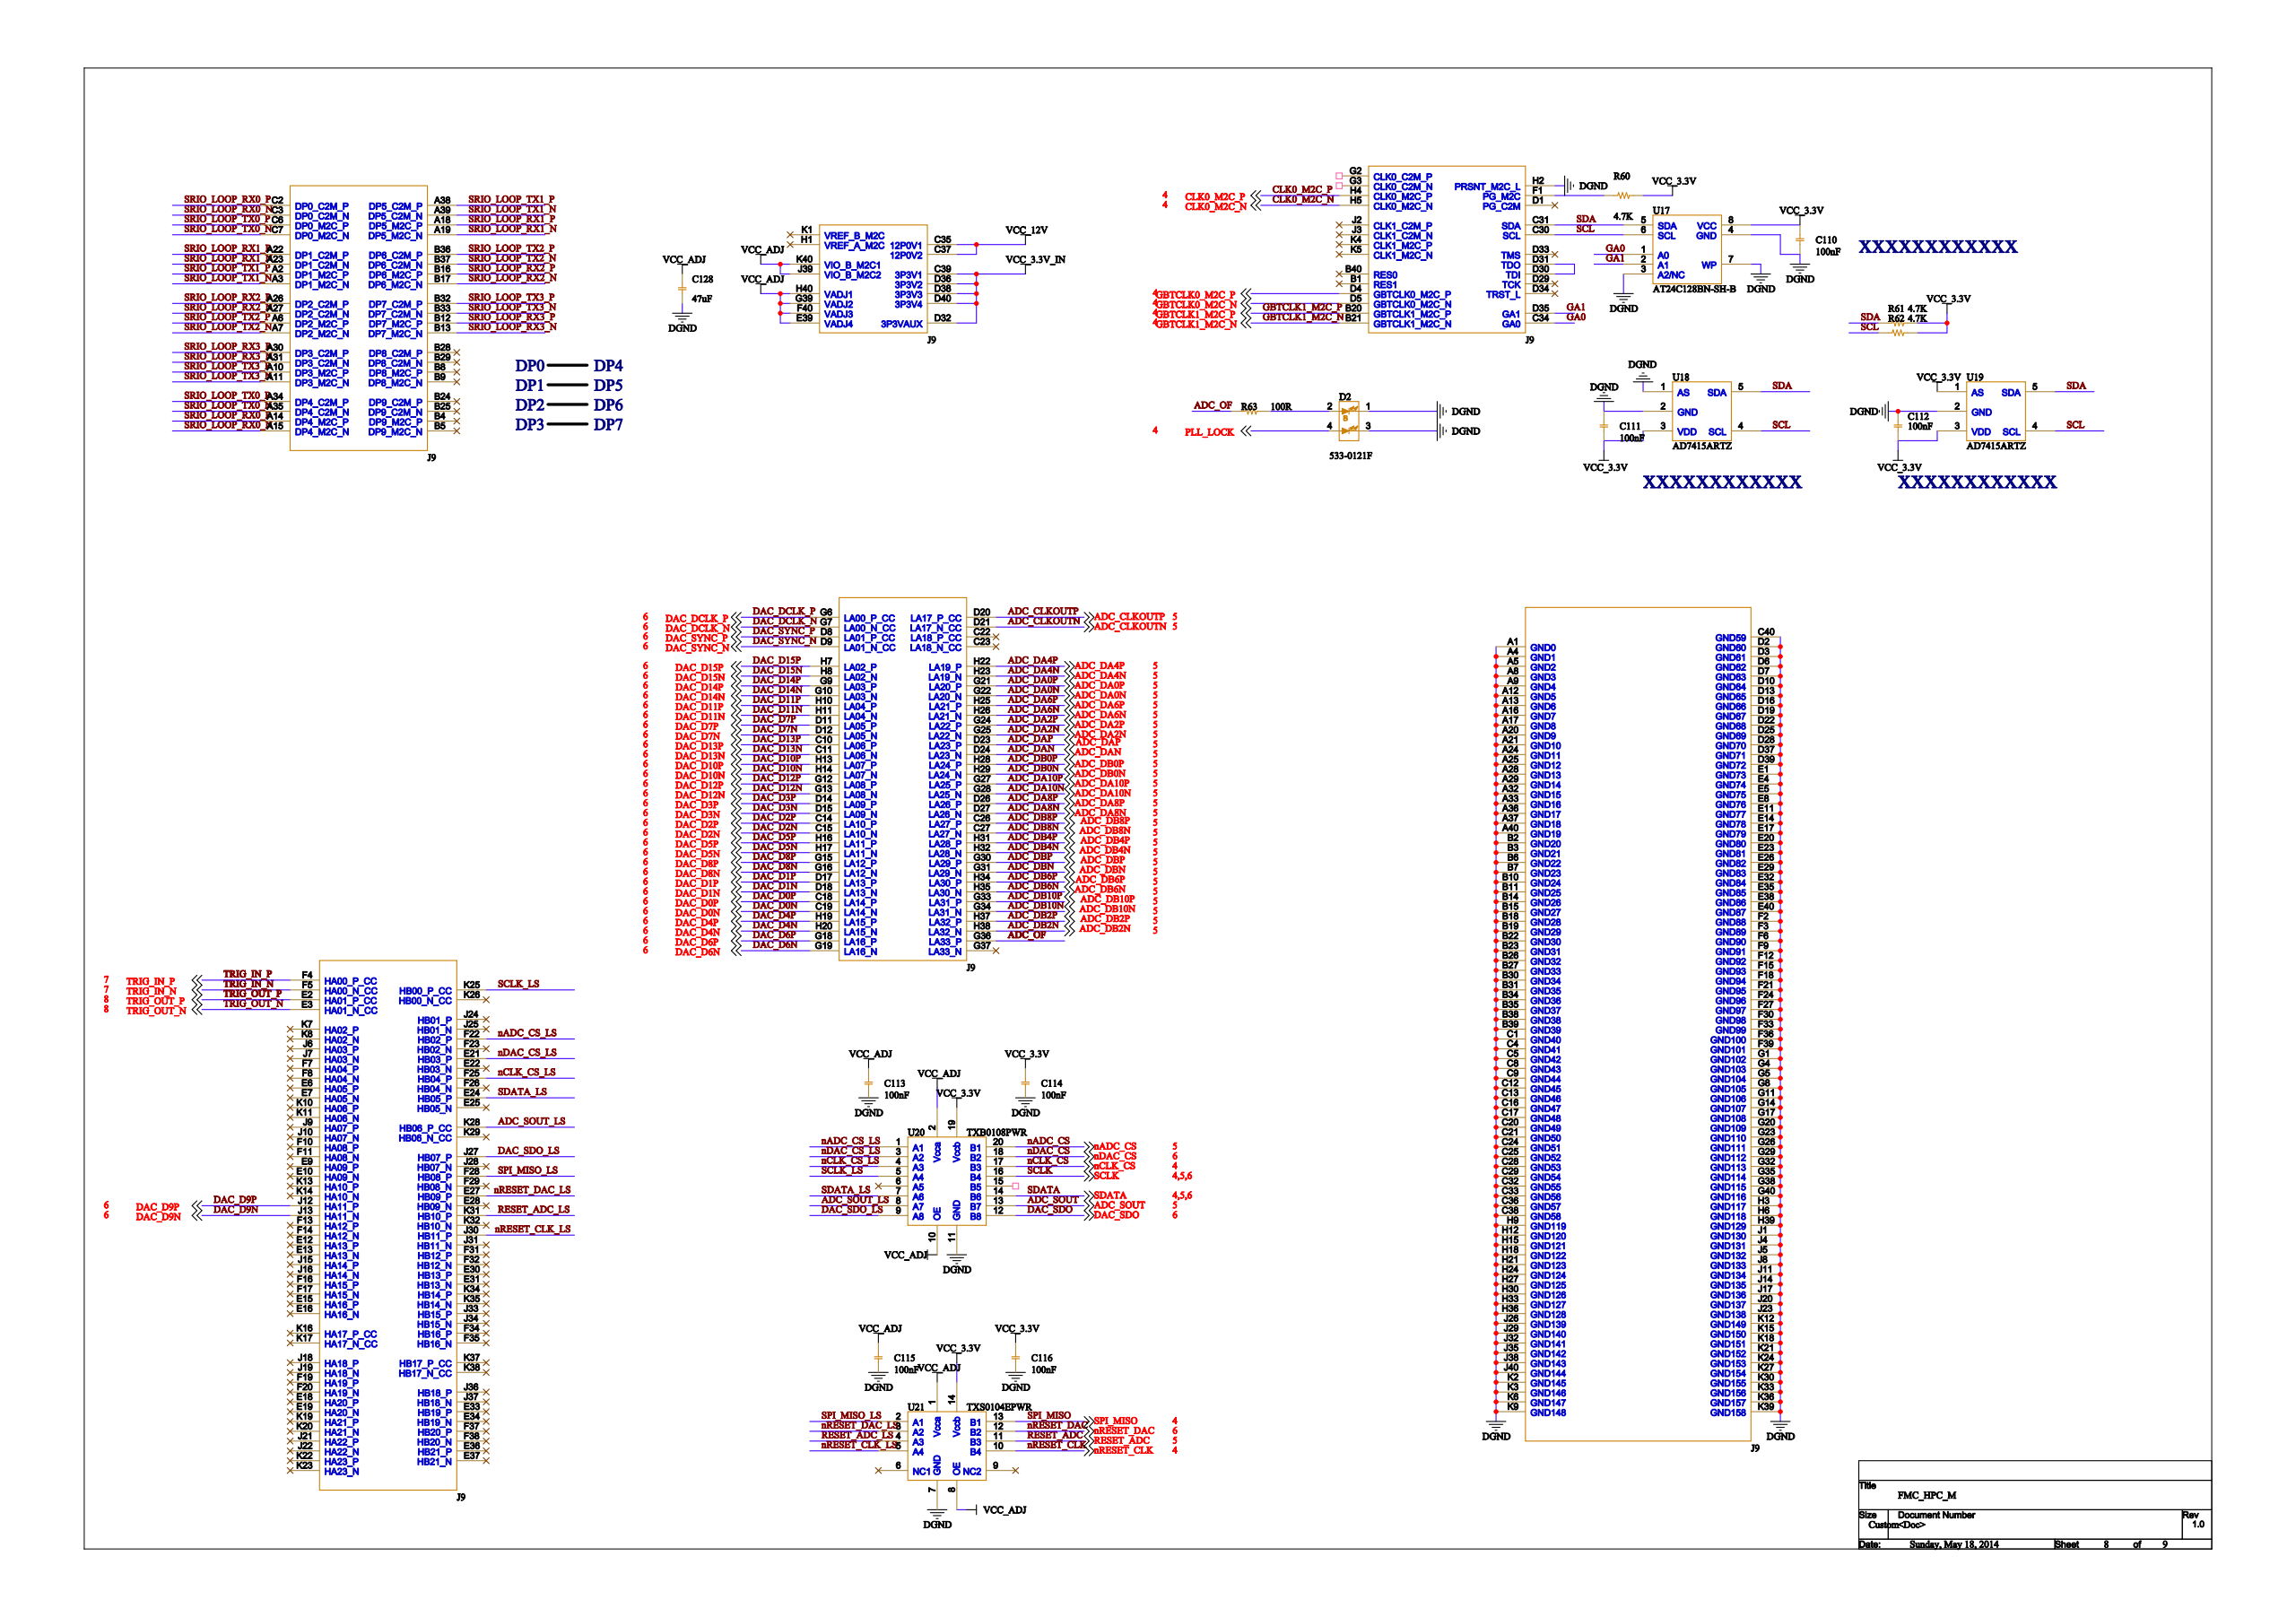Circuit board | Cadence Allegro | 233 parts | 224 nets | one sheet of the schematic
Parts on this sheet (reference | value | footprint):
C110 | 100nF | FPC-0402C
C111 | 100nF | FPC-0402C
C112 | 100nF | FPC-0402C
C113 | 100nF | FPC-0402C
C114 | 100nF | FPC-0402C
C115 | 100nF | FPC-0402C
C116 | 100nF | FPC-0402C
C128 | 47uF | FPC-1206C
D2 | 533-0121F | FPC-LED4-4R3X8R1-1R1-1
J9 | ASP-134485-01 | FPC-CON90VP1R27-10X40SM
R60 | 4.7K | FPC-0603R
R61 | 4.7K | FPC-0603R
R62 | 4.7K | FPC-0603R
R63 | 100R | FPC-0603R
U17 | AT24C128BN-SH-B | FPC-SO8-150
U18 | AD7415ARTZ | FPC-SOT23-6
U19 | AD7415ARTZ | FPC-SOT23-6
U20 | TXB0108PWR | FPC-TSSOP20-0R65-4R40
U21 | TXS0104EPWR | FPC-TSSOP14-0R65-4R40
Nets of these parts (net: part-pin ...):
DGND: C110-1 C111-2 C112-2 C113-1 C114-1 C115-1 C116-1 C128-2 D2-1 D2-3 U17-3 U17-4 U17-7 U18-1 U18-2 U19-2 U20-11 U21-7 J9-A1 J9-A4 J9-A5 J9-A8 J9-A9 J9-A12 J9-A13 J9-A16 J9-A17 J9-A20 J9-A21 J9-A24 J9-A25 J9-A28 J9-A29 J9-A32 J9-A33 J9-A36 J9-A37 J9-A40 J9-B2 J9-B3 J9-B6 J9-B7 J9-B10 J9-B11 J9-B14 J9-B15 J9-B18 J9-B19 J9-B22 J9-B23 J9-B26 J9-B27 J9-B30 J9-B31 J9-B34 J9-B35 J9-B38 J9-B39 J9-C1 J9-C4 J9-C5 J9-C8 J9-C9 J9-C12 J9-C13 J9-C16 J9-C17 J9-C20 J9-C21 J9-C24 J9-C25 J9-C28 J9-C29 J9-C32 J9-C33 J9-C36 J9-C38 J9-C40 J9-D2 J9-D3 J9-D6 J9-D7 J9-D10 J9-D13 J9-D16 J9-D19 J9-D22 J9-D25 J9-D28 J9-D37 J9-D39 J9-E1 J9-E4 J9-E5 J9-E8 J9-E11 J9-E14 J9-E17 J9-E20 J9-E23 J9-E26 J9-E29 J9-E32 J9-E35 J9-E38 J9-E40 J9-F2 J9-F3 J9-F6 J9-F9 J9-F12 J9-F15 J9-F18 J9-F21 J9-F24 J9-F27 J9-F30 J9-F33 J9-F36 J9-F39 J9-G1 J9-G4 J9-G5 J9-G8 J9-G11 J9-G14 J9-G17 J9-G20 J9-G23 J9-G26 J9-G29 J9-G32 J9-G35 J9-G38 J9-G40 J9-H2 J9-H3 J9-H6 J9-H9 J9-H12 J9-H15 J9-H18 J9-H21 J9-H24 J9-H27 J9-H30 J9-H33 J9-H36 J9-H39 J9-J1 J9-J4 J9-J5 J9-J8 J9-J11 J9-J14 J9-J17 J9-J20 J9-J23 J9-J26 J9-J29 J9-J32 J9-J35 J9-J38 J9-J40 J9-K2 J9-K3 J9-K6 J9-K9 J9-K12 J9-K15 J9-K18 J9-K21 J9-K24 J9-K27 J9-K30 J9-K33 J9-K36 J9-K39
VCC_3.3V: C110-2 C111-1 C112-1 C114-2 C116-2 R60-2 R61-1 R62-1 U17-8 U18-3 U19-1 U19-3 U20-19 U21-14
VCC_ADJ: C113-2 C115-2 C128-1 U20-2 U20-10 U21-1 U21-8 J9-E39 J9-F40 J9-G39 J9-H40 J9-J39 J9-K40
VCC_3.3V_IN: J9-C39 J9-D32 J9-D36 J9-D38 J9-D40
NRESET_DAC: U21-12
DAC_DCLK_P: J9-G6
DAC_DCLK_N: J9-G7
N413814: D2-2 R63-1
PLL_LOCK: D2-4
SRIO_LOOP_RX0_N: J9-A15 J9-C3
SRIO_LOOP_RX0_P: J9-A14 J9-C2
SRIO_LOOP_TX0_N: J9-A35 J9-C7
SRIO_LOOP_TX0_P: J9-A34 J9-C6
SRIO_LOOP_RX1_N: J9-A19 J9-A23
SRIO_LOOP_RX1_P: J9-A18 J9-A22
SRIO_LOOP_TX1_N: J9-A3 J9-A39
SRIO_LOOP_TX1_P: J9-A2 J9-A38
SRIO_LOOP_RX2_N: J9-A27 J9-B17
SRIO_LOOP_RX2_P: J9-A26 J9-B16
SRIO_LOOP_TX2_N: J9-A7 J9-B37
SRIO_LOOP_TX2_P: J9-A6 J9-B36
SRIO_LOOP_RX3_N: J9-A31 J9-B13
SRIO_LOOP_RX3_P: J9-A30 J9-B12
SRIO_LOOP_TX3_N: J9-A11 J9-B33
SRIO_LOOP_TX3_P: J9-A10 J9-B32
TRIG_IN_N: J9-F5
TRIG_IN_P: J9-F4
TRIG_OUT_N: J9-E3
TRIG_OUT_P: J9-E2
DAC_D9N: J9-J13
DAC_D9P: J9-J12
SCLK_LS: U20-5 J9-K25
NADC_CS_LS: U20-1 J9-F22
NDAC_CS_LS: U20-3 J9-E21
NCLK_CS_LS: U20-4 J9-F25
SDATA_LS: U20-7 J9-E24
ADC_SOUT_LS: U20-8 J9-K28
DAC_SDO_LS: U20-9 J9-J27
SPI_MISO_LS: U21-2 J9-F28
NRESET_DAC_LS: U21-3 J9-E27
RESET_ADC_LS: U21-4 J9-K31
NRESET_CLK_LS: U21-5 J9-J30
DAC_SYNC_N: J9-D9
DAC_SYNC_P: J9-D8
DAC_D15N: J9-H8
DAC_D15P: J9-H7
DAC_D14N: J9-G10
DAC_D14P: J9-G9
DAC_D11N: J9-H11
DAC_D11P: J9-H10
DAC_D7N: J9-D12
DAC_D7P: J9-D11
DAC_D13N: J9-C11
DAC_D13P: J9-C10
DAC_D10N: J9-H14
DAC_D10P: J9-H13
DAC_D12N: J9-G13
DAC_D12P: J9-G12
DAC_D3N: J9-D15
DAC_D3P: J9-D14
DAC_D2N: J9-C15
DAC_D2P: J9-C14
DAC_D5N: J9-H17
DAC_D5P: J9-H16
DAC_D8N: J9-G16
DAC_D8P: J9-G15
DAC_D1N: J9-D18
DAC_D1P: J9-D17
DAC_D0N: J9-C19
DAC_D0P: J9-C18
DAC_D4N: J9-H20
DAC_D4P: J9-H19
DAC_D6N: J9-G19
DAC_D6P: J9-G18
ADC_CLKOUTN: J9-D21
ADC_CLKOUTP: J9-D20
ADC_DA4N: J9-H23
ADC_DA4P: J9-H22
ADC_DA0N: J9-G22
ADC_DA0P: J9-G21
ADC_DA6N: J9-H26
ADC_DA6P: J9-H25
ADC_DA2N: J9-G25
ADC_DA2P: J9-G24
ADC_DAN: J9-D24
ADC_DAP: J9-D23
ADC_DB0N: J9-H29
ADC_DB0P: J9-H28
ADC_DA10N: J9-G28
ADC_DA10P: J9-G27
ADC_DA8N: J9-D27
ADC_DA8P: J9-D26
ADC_DB8N: J9-C27
ADC_DB8P: J9-C26
ADC_DB4N: J9-H32
ADC_DB4P: J9-H31
ADC_DBN: J9-G31
ADC_DBP: J9-G30
ADC_DB6N: J9-H35
ADC_DB6P: J9-H34
ADC_DB10N: J9-G34
ADC_DB10P: J9-G33
ADC_DB2N: J9-H38
ADC_DB2P: J9-H37
ADC_OF: R63-2 J9-G36
VCC_12V: J9-C35 J9-C37
CLK0_M2C_N: J9-H5
CLK0_M2C_P: J9-H4
GA0: U17-1 J9-C34
GA1: U17-2 J9-D35
GBTCLK0_M2C_N: J9-D5
GBTCLK0_M2C_P: J9-D4
GBTCLK1_M2C_N: J9-B21
GBTCLK1_M2C_P: J9-B20
N17048: R60-1 J9-F1
SCL: R62-2 U17-6 U18-4 U19-4 J9-C30
SDA: R61-2 U17-5 U18-5 U19-5 J9-C31
NRESET_CLK: U21-10
RESET_ADC: U21-11
SPI_MISO: U21-13
SCLK: U20-16
SDATA: U20-14
ADC_SOUT: U20-13
NADC_CS: U20-20
NDAC_CS: U20-18
DAC_SDO: U20-12
NCLK_CS: U20-17